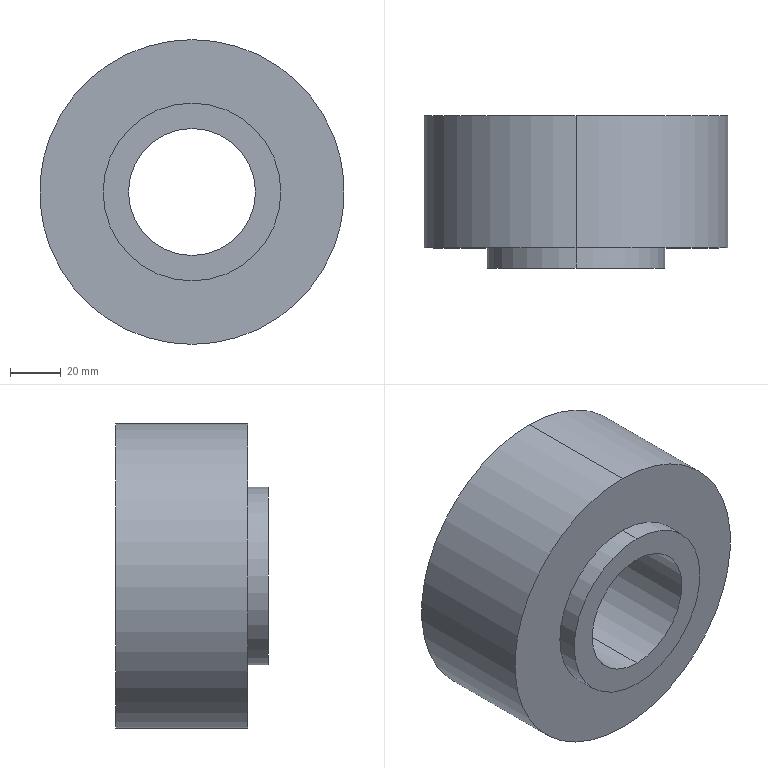Part | SolidWorks | features Revolution 1 | 1 solid | 9 faces | box 120 x 60 x 120 mm | volume 501084 mm3 | cylinder 6 | plane 3 | commonest cylinder face diameters 50 x2 70 x2 120 x2
STEP:
#1=CARTESIAN_POINT('',(0.,8.,-35.));
#2=VERTEX_POINT('',#1);
#3=CARTESIAN_POINT('',(0.,8.,35.));
#4=VERTEX_POINT('',#3);
#5=CARTESIAN_POINT('',(0.,8.,0.));
#6=DIRECTION('',(0.,-1.,0.));
#7=DIRECTION('',(0.,0.,-1.));
#8=AXIS2_PLACEMENT_3D('',#5,#6,#7);
#9=CIRCLE('',#8,35.);
#10=EDGE_CURVE('',#2,#4,#9,.T.);
#11=ORIENTED_EDGE('',*,*,#10,.T.);
#12=CARTESIAN_POINT('',(0.,0.,35.));
#13=VERTEX_POINT('',#12);
#14=CARTESIAN_POINT('',(0.,0.,35.));
#15=DIRECTION('',(0.,-1.,0.));
#16=VECTOR('',#15,1000.);
#17=LINE('',#14,#16);
#18=EDGE_CURVE('',#4,#13,#17,.T.);
#19=ORIENTED_EDGE('',*,*,#18,.T.);
#20=CARTESIAN_POINT('',(0.,0.,-35.));
#21=VERTEX_POINT('',#20);
#22=CARTESIAN_POINT('',(0.,0.,0.));
#23=DIRECTION('',(0.,-1.,0.));
#24=DIRECTION('',(0.,0.,-1.));
#25=AXIS2_PLACEMENT_3D('',#22,#23,#24);
#26=CIRCLE('',#25,35.);
#27=EDGE_CURVE('',#21,#13,#26,.T.);
#28=ORIENTED_EDGE('',*,*,#27,.F.);
#29=CARTESIAN_POINT('',(0.,0.,-35.));
#30=DIRECTION('',(0.,-1.,0.));
#31=VECTOR('',#30,1000.);
#32=LINE('',#29,#31);
#33=EDGE_CURVE('',#2,#21,#32,.T.);
#34=ORIENTED_EDGE('',*,*,#33,.F.);
#35=EDGE_LOOP('',(#11,#19,#28,#34));
#36=FACE_OUTER_BOUND('',#35,.T.);
#37=CARTESIAN_POINT('',(0.,0.,0.));
#38=DIRECTION('',(0.,-1.,0.));
#39=DIRECTION('',(0.,0.,-1.));
#40=AXIS2_PLACEMENT_3D('',#37,#38,#39);
#41=CYLINDRICAL_SURFACE('',#40,35.);
#42=ADVANCED_FACE('',(#36),#41,.T.);
#43=CARTESIAN_POINT('',(0.,60.,-60.));
#44=VERTEX_POINT('',#43);
#45=CARTESIAN_POINT('',(0.,60.,60.));
#46=VERTEX_POINT('',#45);
#47=CARTESIAN_POINT('',(0.,60.,0.));
#48=DIRECTION('',(0.,-1.,0.));
#49=DIRECTION('',(0.,0.,-1.));
#50=AXIS2_PLACEMENT_3D('',#47,#48,#49);
#51=CIRCLE('',#50,60.);
#52=EDGE_CURVE('',#44,#46,#51,.T.);
#53=ORIENTED_EDGE('',*,*,#52,.T.);
#54=CARTESIAN_POINT('',(0.,8.,60.));
#55=VERTEX_POINT('',#54);
#56=CARTESIAN_POINT('',(0.,0.,60.));
#57=DIRECTION('',(0.,-1.,0.));
#58=VECTOR('',#57,1000.);
#59=LINE('',#56,#58);
#60=EDGE_CURVE('',#46,#55,#59,.T.);
#61=ORIENTED_EDGE('',*,*,#60,.T.);
#62=CARTESIAN_POINT('',(0.,8.,-60.));
#63=VERTEX_POINT('',#62);
#64=CARTESIAN_POINT('',(0.,8.,0.));
#65=DIRECTION('',(0.,-1.,0.));
#66=DIRECTION('',(0.,0.,-1.));
#67=AXIS2_PLACEMENT_3D('',#64,#65,#66);
#68=CIRCLE('',#67,60.);
#69=EDGE_CURVE('',#63,#55,#68,.T.);
#70=ORIENTED_EDGE('',*,*,#69,.F.);
#71=CARTESIAN_POINT('',(0.,0.,-60.));
#72=DIRECTION('',(0.,-1.,0.));
#73=VECTOR('',#72,1000.);
#74=LINE('',#71,#73);
#75=EDGE_CURVE('',#44,#63,#74,.T.);
#76=ORIENTED_EDGE('',*,*,#75,.F.);
#77=EDGE_LOOP('',(#53,#61,#70,#76));
#78=FACE_OUTER_BOUND('',#77,.T.);
#79=CARTESIAN_POINT('',(0.,0.,0.));
#80=DIRECTION('',(0.,-1.,0.));
#81=DIRECTION('',(0.,0.,-1.));
#82=AXIS2_PLACEMENT_3D('',#79,#80,#81);
#83=CYLINDRICAL_SURFACE('',#82,60.);
#84=ADVANCED_FACE('',(#78),#83,.T.);
#85=CARTESIAN_POINT('',(0.,60.,25.));
#86=VERTEX_POINT('',#85);
#87=CARTESIAN_POINT('',(0.,60.,-25.));
#88=VERTEX_POINT('',#87);
#89=CARTESIAN_POINT('',(0.,60.,0.));
#90=DIRECTION('',(0.,-1.,0.));
#91=DIRECTION('',(0.,0.,-1.));
#92=AXIS2_PLACEMENT_3D('',#89,#90,#91);
#93=CIRCLE('',#92,25.);
#94=EDGE_CURVE('',#86,#88,#93,.T.);
#95=ORIENTED_EDGE('',*,*,#94,.F.);
#96=CARTESIAN_POINT('',(0.,0.,25.));
#97=VERTEX_POINT('',#96);
#98=CARTESIAN_POINT('',(0.,0.,25.));
#99=DIRECTION('',(0.,-1.,0.));
#100=VECTOR('',#99,1000.);
#101=LINE('',#98,#100);
#102=EDGE_CURVE('',#86,#97,#101,.T.);
#103=ORIENTED_EDGE('',*,*,#102,.T.);
#104=CARTESIAN_POINT('',(0.,0.,-25.));
#105=VERTEX_POINT('',#104);
#106=CARTESIAN_POINT('',(0.,0.,0.));
#107=DIRECTION('',(0.,-1.,0.));
#108=DIRECTION('',(0.,0.,-1.));
#109=AXIS2_PLACEMENT_3D('',#106,#107,#108);
#110=CIRCLE('',#109,25.);
#111=EDGE_CURVE('',#97,#105,#110,.T.);
#112=ORIENTED_EDGE('',*,*,#111,.T.);
#113=CARTESIAN_POINT('',(0.,0.,-25.));
#114=DIRECTION('',(0.,-1.,0.));
#115=VECTOR('',#114,1000.);
#116=LINE('',#113,#115);
#117=EDGE_CURVE('',#88,#105,#116,.T.);
#118=ORIENTED_EDGE('',*,*,#117,.F.);
#119=EDGE_LOOP('',(#95,#103,#112,#118));
#120=FACE_OUTER_BOUND('',#119,.T.);
#121=CARTESIAN_POINT('',(0.,0.,0.));
#122=DIRECTION('',(0.,-1.,0.));
#123=DIRECTION('',(0.,0.,-1.));
#124=AXIS2_PLACEMENT_3D('',#121,#122,#123);
#125=CYLINDRICAL_SURFACE('',#124,25.);
#126=ADVANCED_FACE('',(#120),#125,.F.);
#127=ORIENTED_EDGE('',*,*,#27,.T.);
#128=CARTESIAN_POINT('',(0.,0.,0.));
#129=DIRECTION('',(0.,-1.,0.));
#130=DIRECTION('',(0.,0.,-1.));
#131=AXIS2_PLACEMENT_3D('',#128,#129,#130);
#132=CIRCLE('',#131,35.);
#133=EDGE_CURVE('',#13,#21,#132,.T.);
#134=ORIENTED_EDGE('',*,*,#133,.T.);
#135=EDGE_LOOP('',(#127,#134));
#136=FACE_OUTER_BOUND('',#135,.T.);
#137=CARTESIAN_POINT('',(0.,0.,0.));
#138=DIRECTION('',(0.,-1.,0.));
#139=DIRECTION('',(0.,0.,-1.));
#140=AXIS2_PLACEMENT_3D('',#137,#138,#139);
#141=CIRCLE('',#140,25.);
#142=EDGE_CURVE('',#105,#97,#141,.T.);
#143=ORIENTED_EDGE('',*,*,#142,.F.);
#144=ORIENTED_EDGE('',*,*,#111,.F.);
#145=EDGE_LOOP('',(#143,#144));
#146=FACE_BOUND('',#145,.T.);
#147=CARTESIAN_POINT('',(35.,0.,0.));
#148=DIRECTION('',(0.,-1.,0.));
#149=DIRECTION('',(0.,0.,-1.));
#150=AXIS2_PLACEMENT_3D('',#147,#148,#149);
#151=PLANE('',#150);
#152=ADVANCED_FACE('',(#136,#146),#151,.T.);
#153=ORIENTED_EDGE('',*,*,#102,.F.);
#154=CARTESIAN_POINT('',(0.,60.,0.));
#155=DIRECTION('',(0.,-1.,0.));
#156=DIRECTION('',(0.,0.,-1.));
#157=AXIS2_PLACEMENT_3D('',#154,#155,#156);
#158=CIRCLE('',#157,25.);
#159=EDGE_CURVE('',#88,#86,#158,.T.);
#160=ORIENTED_EDGE('',*,*,#159,.F.);
#161=ORIENTED_EDGE('',*,*,#117,.T.);
#162=ORIENTED_EDGE('',*,*,#142,.T.);
#163=EDGE_LOOP('',(#153,#160,#161,#162));
#164=FACE_OUTER_BOUND('',#163,.T.);
#165=CARTESIAN_POINT('',(0.,0.,0.));
#166=DIRECTION('',(0.,-1.,0.));
#167=DIRECTION('',(0.,0.,-1.));
#168=AXIS2_PLACEMENT_3D('',#165,#166,#167);
#169=CYLINDRICAL_SURFACE('',#168,25.);
#170=ADVANCED_FACE('',(#164),#169,.F.);
#171=ORIENTED_EDGE('',*,*,#159,.T.);
#172=ORIENTED_EDGE('',*,*,#94,.T.);
#173=EDGE_LOOP('',(#171,#172));
#174=FACE_BOUND('',#173,.T.);
#175=ORIENTED_EDGE('',*,*,#52,.F.);
#176=CARTESIAN_POINT('',(0.,60.,0.));
#177=DIRECTION('',(0.,-1.,0.));
#178=DIRECTION('',(0.,0.,-1.));
#179=AXIS2_PLACEMENT_3D('',#176,#177,#178);
#180=CIRCLE('',#179,60.);
#181=EDGE_CURVE('',#46,#44,#180,.T.);
#182=ORIENTED_EDGE('',*,*,#181,.F.);
#183=EDGE_LOOP('',(#175,#182));
#184=FACE_OUTER_BOUND('',#183,.T.);
#185=CARTESIAN_POINT('',(25.,60.,0.));
#186=DIRECTION('',(0.,1.,0.));
#187=DIRECTION('',(0.,0.,1.));
#188=AXIS2_PLACEMENT_3D('',#185,#186,#187);
#189=PLANE('',#188);
#190=ADVANCED_FACE('',(#174,#184),#189,.T.);
#191=ORIENTED_EDGE('',*,*,#60,.F.);
#192=ORIENTED_EDGE('',*,*,#181,.T.);
#193=ORIENTED_EDGE('',*,*,#75,.T.);
#194=CARTESIAN_POINT('',(0.,8.,0.));
#195=DIRECTION('',(0.,-1.,0.));
#196=DIRECTION('',(0.,0.,-1.));
#197=AXIS2_PLACEMENT_3D('',#194,#195,#196);
#198=CIRCLE('',#197,60.);
#199=EDGE_CURVE('',#55,#63,#198,.T.);
#200=ORIENTED_EDGE('',*,*,#199,.F.);
#201=EDGE_LOOP('',(#191,#192,#193,#200));
#202=FACE_OUTER_BOUND('',#201,.T.);
#203=CARTESIAN_POINT('',(0.,0.,0.));
#204=DIRECTION('',(0.,-1.,0.));
#205=DIRECTION('',(0.,0.,-1.));
#206=AXIS2_PLACEMENT_3D('',#203,#204,#205);
#207=CYLINDRICAL_SURFACE('',#206,60.);
#208=ADVANCED_FACE('',(#202),#207,.T.);
#209=ORIENTED_EDGE('',*,*,#69,.T.);
#210=ORIENTED_EDGE('',*,*,#199,.T.);
#211=EDGE_LOOP('',(#209,#210));
#212=FACE_OUTER_BOUND('',#211,.T.);
#213=ORIENTED_EDGE('',*,*,#10,.F.);
#214=CARTESIAN_POINT('',(0.,8.,0.));
#215=DIRECTION('',(0.,-1.,0.));
#216=DIRECTION('',(0.,0.,-1.));
#217=AXIS2_PLACEMENT_3D('',#214,#215,#216);
#218=CIRCLE('',#217,35.);
#219=EDGE_CURVE('',#4,#2,#218,.T.);
#220=ORIENTED_EDGE('',*,*,#219,.F.);
#221=EDGE_LOOP('',(#213,#220));
#222=FACE_BOUND('',#221,.T.);
#223=CARTESIAN_POINT('',(60.,8.,0.));
#224=DIRECTION('',(0.,-1.,0.));
#225=DIRECTION('',(0.,0.,-1.));
#226=AXIS2_PLACEMENT_3D('',#223,#224,#225);
#227=PLANE('',#226);
#228=ADVANCED_FACE('',(#212,#222),#227,.T.);
#229=ORIENTED_EDGE('',*,*,#18,.F.);
#230=ORIENTED_EDGE('',*,*,#219,.T.);
#231=ORIENTED_EDGE('',*,*,#33,.T.);
#232=ORIENTED_EDGE('',*,*,#133,.F.);
#233=EDGE_LOOP('',(#229,#230,#231,#232));
#234=FACE_OUTER_BOUND('',#233,.T.);
#235=CARTESIAN_POINT('',(0.,0.,0.));
#236=DIRECTION('',(0.,-1.,0.));
#237=DIRECTION('',(0.,0.,-1.));
#238=AXIS2_PLACEMENT_3D('',#235,#236,#237);
#239=CYLINDRICAL_SURFACE('',#238,35.);
#240=ADVANCED_FACE('',(#234),#239,.T.);
#241=CLOSED_SHELL('',(#42,#84,#126,#152,#170,#190,#208,#228,#240));
#242=MANIFOLD_SOLID_BREP('',#241);
#243=CARTESIAN_POINT('',(0.,0.,0.));
#244=DIRECTION('',(0.,0.,1.));
#245=DIRECTION('',(1.,0.,0.));
#246=AXIS2_PLACEMENT_3D('',#243,#244,#245);
#247=(LENGTH_UNIT()NAMED_UNIT(*)SI_UNIT(.MILLI.,.METRE.));
#248=UNCERTAINTY_MEASURE_WITH_UNIT(LENGTH_MEASURE(0.00001),#247,'','');
#249=(NAMED_UNIT(*)PLANE_ANGLE_UNIT()SI_UNIT($,.RADIAN.));
#250=(NAMED_UNIT(*)SI_UNIT($,.STERADIAN.)SOLID_ANGLE_UNIT());
#251=(GEOMETRIC_REPRESENTATION_CONTEXT(3)GLOBAL_UNCERTAINTY_ASSIGNED_CONTEXT((#248))GLOBAL_UNIT_ASSIGNED_CONTEXT((#247,#249,#250))REPRESENTATION_CONTEXT('',''));
#252=ADVANCED_BREP_SHAPE_REPRESENTATION('',(#242,#246),#251);